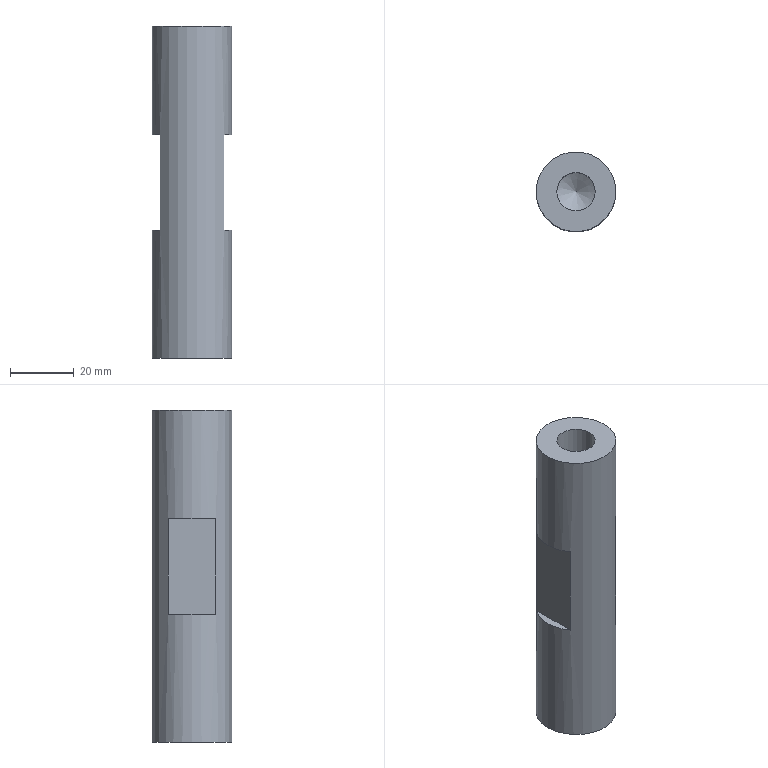Part | NX | features solid 2 | 1 solid | 13 faces | box 25 x 25 x 104 mm | volume 43591 mm3 | plane 8 | cylinder 3 | cone 2 | commonest cylinder face diameters 12 x2 25 x1
STEP:
#1=CARTESIAN_POINT('',(-537.5,-40.,-65.));
#2=VERTEX_POINT('',#1);
#3=CARTESIAN_POINT('',(-525.,-40.,-65.));
#4=DIRECTION('',(0.,0.,-1.));
#5=DIRECTION('',(-1.,0.,0.));
#6=AXIS2_PLACEMENT_3D('',#3,#4,#5);
#7=CIRCLE('',#6,12.5);
#8=EDGE_CURVE('',#2,#2,#7,.F.);
#9=ORIENTED_EDGE('',*,*,#8,.F.);
#10=EDGE_LOOP('',(#9));
#11=FACE_BOUND('',#10,.T.);
#12=CARTESIAN_POINT('',(-512.5,-40.,-169.));
#13=VERTEX_POINT('',#12);
#14=CARTESIAN_POINT('',(-525.,-40.,-169.));
#15=DIRECTION('',(0.,0.,1.));
#16=DIRECTION('',(1.,0.,0.));
#17=AXIS2_PLACEMENT_3D('',#14,#15,#16);
#18=CIRCLE('',#17,12.5);
#19=EDGE_CURVE('',#13,#13,#18,.T.);
#20=ORIENTED_EDGE('',*,*,#19,.T.);
#21=EDGE_LOOP('',(#20));
#22=FACE_BOUND('',#21,.T.);
#23=CARTESIAN_POINT('',(-515.,-47.5,-99.));
#24=VERTEX_POINT('',#23);
#25=CARTESIAN_POINT('',(-515.,-47.5,-129.));
#26=VERTEX_POINT('',#25);
#27=CARTESIAN_POINT('',(-515.,-47.5,-169.));
#28=DIRECTION('',(0.,0.,1.));
#29=VECTOR('',#28,1000.);
#30=LINE('',#27,#29);
#31=EDGE_CURVE('',#24,#26,#30,.F.);
#32=ORIENTED_EDGE('',*,*,#31,.F.);
#33=CARTESIAN_POINT('',(-515.,-32.5,-99.));
#34=VERTEX_POINT('',#33);
#35=CARTESIAN_POINT('',(-525.,-40.,-99.));
#36=DIRECTION('',(0.,0.,-1.));
#37=DIRECTION('',(-1.,0.,0.));
#38=AXIS2_PLACEMENT_3D('',#35,#36,#37);
#39=CIRCLE('',#38,12.5);
#40=EDGE_CURVE('',#34,#24,#39,.T.);
#41=ORIENTED_EDGE('',*,*,#40,.F.);
#42=CARTESIAN_POINT('',(-515.,-32.5,-129.));
#43=VERTEX_POINT('',#42);
#44=CARTESIAN_POINT('',(-515.,-32.5,-169.));
#45=DIRECTION('',(0.,0.,1.));
#46=VECTOR('',#45,1000.);
#47=LINE('',#44,#46);
#48=EDGE_CURVE('',#43,#34,#47,.T.);
#49=ORIENTED_EDGE('',*,*,#48,.F.);
#50=CARTESIAN_POINT('',(-525.,-40.,-129.));
#51=DIRECTION('',(0.,0.,-1.));
#52=DIRECTION('',(-1.,0.,0.));
#53=AXIS2_PLACEMENT_3D('',#50,#51,#52);
#54=CIRCLE('',#53,12.5);
#55=EDGE_CURVE('',#26,#43,#54,.F.);
#56=ORIENTED_EDGE('',*,*,#55,.F.);
#57=EDGE_LOOP('',(#32,#41,#49,#56));
#58=FACE_BOUND('',#57,.T.);
#59=CARTESIAN_POINT('',(-535.,-32.5,-99.));
#60=VERTEX_POINT('',#59);
#61=CARTESIAN_POINT('',(-535.,-47.5,-99.));
#62=VERTEX_POINT('',#61);
#63=CARTESIAN_POINT('',(-525.,-40.,-99.));
#64=DIRECTION('',(0.,0.,-1.));
#65=DIRECTION('',(-1.,0.,0.));
#66=AXIS2_PLACEMENT_3D('',#63,#64,#65);
#67=CIRCLE('',#66,12.5);
#68=EDGE_CURVE('',#60,#62,#67,.F.);
#69=ORIENTED_EDGE('',*,*,#68,.T.);
#70=CARTESIAN_POINT('',(-535.,-47.5,-129.));
#71=VERTEX_POINT('',#70);
#72=CARTESIAN_POINT('',(-535.,-47.5,-99.));
#73=DIRECTION('',(0.,0.,1.));
#74=VECTOR('',#73,1000.);
#75=LINE('',#72,#74);
#76=EDGE_CURVE('',#62,#71,#75,.F.);
#77=ORIENTED_EDGE('',*,*,#76,.T.);
#78=CARTESIAN_POINT('',(-535.,-32.5,-129.));
#79=VERTEX_POINT('',#78);
#80=CARTESIAN_POINT('',(-525.,-40.,-129.));
#81=DIRECTION('',(0.,0.,-1.));
#82=DIRECTION('',(-1.,0.,0.));
#83=AXIS2_PLACEMENT_3D('',#80,#81,#82);
#84=CIRCLE('',#83,12.5);
#85=EDGE_CURVE('',#71,#79,#84,.T.);
#86=ORIENTED_EDGE('',*,*,#85,.T.);
#87=CARTESIAN_POINT('',(-535.,-32.5,-169.));
#88=DIRECTION('',(0.,0.,1.));
#89=VECTOR('',#88,1000.);
#90=LINE('',#87,#89);
#91=EDGE_CURVE('',#79,#60,#90,.T.);
#92=ORIENTED_EDGE('',*,*,#91,.T.);
#93=EDGE_LOOP('',(#69,#77,#86,#92));
#94=FACE_BOUND('',#93,.T.);
#95=CARTESIAN_POINT('',(-525.,-40.,-169.));
#96=DIRECTION('',(0.,0.,1.));
#97=DIRECTION('',(1.,0.,0.));
#98=AXIS2_PLACEMENT_3D('',#95,#96,#97);
#99=CYLINDRICAL_SURFACE('',#98,12.5);
#100=ADVANCED_FACE('',(#11,#22,#58,#94),#99,.T.);
#101=CARTESIAN_POINT('',(-519.,-40.,-169.));
#102=VERTEX_POINT('',#101);
#103=CARTESIAN_POINT('',(-525.,-40.,-169.));
#104=DIRECTION('',(0.,0.,1.));
#105=DIRECTION('',(1.,0.,0.));
#106=AXIS2_PLACEMENT_3D('',#103,#104,#105);
#107=CIRCLE('',#106,6.);
#108=EDGE_CURVE('',#102,#102,#107,.T.);
#109=ORIENTED_EDGE('',*,*,#108,.T.);
#110=EDGE_LOOP('',(#109));
#111=FACE_BOUND('',#110,.T.);
#112=ORIENTED_EDGE('',*,*,#19,.F.);
#113=EDGE_LOOP('',(#112));
#114=FACE_BOUND('',#113,.T.);
#115=CARTESIAN_POINT('',(-525.,-40.,-169.));
#116=DIRECTION('',(0.,0.,1.));
#117=DIRECTION('',(1.,0.,0.));
#118=AXIS2_PLACEMENT_3D('',#115,#116,#117);
#119=PLANE('',#118);
#120=ADVANCED_FACE('',(#111,#114),#119,.F.);
#121=CARTESIAN_POINT('',(-531.,-40.,-65.));
#122=VERTEX_POINT('',#121);
#123=CARTESIAN_POINT('',(-525.,-40.,-65.));
#124=DIRECTION('',(0.,0.,-1.));
#125=DIRECTION('',(-1.,0.,0.));
#126=AXIS2_PLACEMENT_3D('',#123,#124,#125);
#127=CIRCLE('',#126,6.);
#128=EDGE_CURVE('',#122,#122,#127,.T.);
#129=ORIENTED_EDGE('',*,*,#128,.T.);
#130=EDGE_LOOP('',(#129));
#131=FACE_BOUND('',#130,.T.);
#132=ORIENTED_EDGE('',*,*,#8,.T.);
#133=EDGE_LOOP('',(#132));
#134=FACE_BOUND('',#133,.T.);
#135=CARTESIAN_POINT('',(-610.,110.,-65.));
#136=DIRECTION('',(0.,0.,-1.));
#137=DIRECTION('',(0.,1.,0.));
#138=AXIS2_PLACEMENT_3D('',#135,#136,#137);
#139=PLANE('',#138);
#140=ADVANCED_FACE('',(#131,#134),#139,.F.);
#141=CARTESIAN_POINT('',(-531.,-40.,-85.));
#142=VERTEX_POINT('',#141);
#143=CARTESIAN_POINT('',(-525.,-40.,-85.));
#144=DIRECTION('',(0.,0.,-1.));
#145=DIRECTION('',(-1.,0.,0.));
#146=AXIS2_PLACEMENT_3D('',#143,#144,#145);
#147=CIRCLE('',#146,6.);
#148=EDGE_CURVE('',#142,#142,#147,.T.);
#149=ORIENTED_EDGE('',*,*,#148,.F.);
#150=EDGE_LOOP('',(#149));
#151=FACE_BOUND('',#150,.T.);
#152=CARTESIAN_POINT('',(-525.,-40.,-88.605));
#153=VERTEX_POINT('',#152);
#154=VERTEX_LOOP('',#153);
#155=FACE_BOUND('',#154,.T.);
#156=CARTESIAN_POINT('',(-525.,-40.,-85.));
#157=DIRECTION('',(0.,0.,1.));
#158=DIRECTION('',(1.,0.,0.));
#159=AXIS2_PLACEMENT_3D('',#156,#157,#158);
#160=CONICAL_SURFACE('',#159,6.,1.03);
#161=ADVANCED_FACE('',(#151,#155),#160,.F.);
#162=ORIENTED_EDGE('',*,*,#148,.T.);
#163=EDGE_LOOP('',(#162));
#164=FACE_BOUND('',#163,.T.);
#165=ORIENTED_EDGE('',*,*,#128,.F.);
#166=EDGE_LOOP('',(#165));
#167=FACE_BOUND('',#166,.T.);
#168=CARTESIAN_POINT('',(-525.,-40.,-65.));
#169=DIRECTION('',(0.,0.,-1.));
#170=DIRECTION('',(-1.,0.,0.));
#171=AXIS2_PLACEMENT_3D('',#168,#169,#170);
#172=CYLINDRICAL_SURFACE('',#171,6.);
#173=ADVANCED_FACE('',(#164,#167),#172,.F.);
#174=CARTESIAN_POINT('',(-519.,-40.,-139.));
#175=VERTEX_POINT('',#174);
#176=CARTESIAN_POINT('',(-525.,-40.,-139.));
#177=DIRECTION('',(0.,0.,1.));
#178=DIRECTION('',(1.,0.,0.));
#179=AXIS2_PLACEMENT_3D('',#176,#177,#178);
#180=CIRCLE('',#179,6.);
#181=EDGE_CURVE('',#175,#175,#180,.T.);
#182=ORIENTED_EDGE('',*,*,#181,.F.);
#183=EDGE_LOOP('',(#182));
#184=FACE_BOUND('',#183,.T.);
#185=CARTESIAN_POINT('',(-525.,-40.,-135.395));
#186=VERTEX_POINT('',#185);
#187=VERTEX_LOOP('',#186);
#188=FACE_BOUND('',#187,.T.);
#189=CARTESIAN_POINT('',(-525.,-40.,-139.));
#190=DIRECTION('',(0.,0.,-1.));
#191=DIRECTION('',(-1.,0.,0.));
#192=AXIS2_PLACEMENT_3D('',#189,#190,#191);
#193=CONICAL_SURFACE('',#192,6.,1.03);
#194=ADVANCED_FACE('',(#184,#188),#193,.F.);
#195=ORIENTED_EDGE('',*,*,#181,.T.);
#196=EDGE_LOOP('',(#195));
#197=FACE_BOUND('',#196,.T.);
#198=ORIENTED_EDGE('',*,*,#108,.F.);
#199=EDGE_LOOP('',(#198));
#200=FACE_BOUND('',#199,.T.);
#201=CARTESIAN_POINT('',(-525.,-40.,-169.));
#202=DIRECTION('',(0.,0.,1.));
#203=DIRECTION('',(1.,0.,0.));
#204=AXIS2_PLACEMENT_3D('',#201,#202,#203);
#205=CYLINDRICAL_SURFACE('',#204,6.);
#206=ADVANCED_FACE('',(#197,#200),#205,.F.);
#207=ORIENTED_EDGE('',*,*,#55,.T.);
#208=CARTESIAN_POINT('',(-515.,-25.,-129.));
#209=DIRECTION('',(0.,-1.,0.));
#210=VECTOR('',#209,1000.);
#211=LINE('',#208,#210);
#212=EDGE_CURVE('',#43,#26,#211,.T.);
#213=ORIENTED_EDGE('',*,*,#212,.T.);
#214=EDGE_LOOP('',(#207,#213));
#215=FACE_BOUND('',#214,.T.);
#216=CARTESIAN_POINT('',(-525.,-25.,-129.));
#217=DIRECTION('',(0.,0.,-1.));
#218=DIRECTION('',(0.,-1.,0.));
#219=AXIS2_PLACEMENT_3D('',#216,#217,#218);
#220=PLANE('',#219);
#221=ADVANCED_FACE('',(#215),#220,.F.);
#222=ORIENTED_EDGE('',*,*,#40,.T.);
#223=CARTESIAN_POINT('',(-515.,-25.,-99.));
#224=DIRECTION('',(0.,1.,0.));
#225=VECTOR('',#224,1000.);
#226=LINE('',#223,#225);
#227=EDGE_CURVE('',#34,#24,#226,.F.);
#228=ORIENTED_EDGE('',*,*,#227,.F.);
#229=EDGE_LOOP('',(#222,#228));
#230=FACE_BOUND('',#229,.T.);
#231=CARTESIAN_POINT('',(-525.,-25.,-99.));
#232=DIRECTION('',(0.,0.,-1.));
#233=DIRECTION('',(0.,-1.,0.));
#234=AXIS2_PLACEMENT_3D('',#231,#232,#233);
#235=PLANE('',#234);
#236=ADVANCED_FACE('',(#230),#235,.T.);
#237=ORIENTED_EDGE('',*,*,#31,.T.);
#238=ORIENTED_EDGE('',*,*,#212,.F.);
#239=ORIENTED_EDGE('',*,*,#48,.T.);
#240=ORIENTED_EDGE('',*,*,#227,.T.);
#241=EDGE_LOOP('',(#237,#238,#239,#240));
#242=FACE_BOUND('',#241,.T.);
#243=CARTESIAN_POINT('',(-515.,-25.,-129.));
#244=DIRECTION('',(-1.,0.,0.));
#245=DIRECTION('',(0.,0.,1.));
#246=AXIS2_PLACEMENT_3D('',#243,#244,#245);
#247=PLANE('',#246);
#248=ADVANCED_FACE('',(#242),#247,.F.);
#249=CARTESIAN_POINT('',(-535.,-25.,-129.));
#250=DIRECTION('',(0.,1.,0.));
#251=VECTOR('',#250,1000.);
#252=LINE('',#249,#251);
#253=EDGE_CURVE('',#79,#71,#252,.F.);
#254=ORIENTED_EDGE('',*,*,#253,.F.);
#255=ORIENTED_EDGE('',*,*,#85,.F.);
#256=EDGE_LOOP('',(#254,#255));
#257=FACE_BOUND('',#256,.T.);
#258=CARTESIAN_POINT('',(-525.,-25.,-129.));
#259=DIRECTION('',(0.,0.,-1.));
#260=DIRECTION('',(0.,-1.,0.));
#261=AXIS2_PLACEMENT_3D('',#258,#259,#260);
#262=PLANE('',#261);
#263=ADVANCED_FACE('',(#257),#262,.F.);
#264=CARTESIAN_POINT('',(-535.,-25.,-99.));
#265=DIRECTION('',(0.,-1.,0.));
#266=VECTOR('',#265,1000.);
#267=LINE('',#264,#266);
#268=EDGE_CURVE('',#60,#62,#267,.T.);
#269=ORIENTED_EDGE('',*,*,#268,.T.);
#270=ORIENTED_EDGE('',*,*,#68,.F.);
#271=EDGE_LOOP('',(#269,#270));
#272=FACE_BOUND('',#271,.T.);
#273=CARTESIAN_POINT('',(-525.,-25.,-99.));
#274=DIRECTION('',(0.,0.,-1.));
#275=DIRECTION('',(0.,-1.,0.));
#276=AXIS2_PLACEMENT_3D('',#273,#274,#275);
#277=PLANE('',#276);
#278=ADVANCED_FACE('',(#272),#277,.T.);
#279=ORIENTED_EDGE('',*,*,#268,.F.);
#280=ORIENTED_EDGE('',*,*,#91,.F.);
#281=ORIENTED_EDGE('',*,*,#253,.T.);
#282=ORIENTED_EDGE('',*,*,#76,.F.);
#283=EDGE_LOOP('',(#279,#280,#281,#282));
#284=FACE_BOUND('',#283,.T.);
#285=CARTESIAN_POINT('',(-535.,-25.,-129.));
#286=DIRECTION('',(-1.,0.,0.));
#287=DIRECTION('',(0.,0.,1.));
#288=AXIS2_PLACEMENT_3D('',#285,#286,#287);
#289=PLANE('',#288);
#290=ADVANCED_FACE('',(#284),#289,.T.);
#291=CLOSED_SHELL('',(#100,#120,#140,#161,#173,#194,#206,#221,#236,#248,#263,#278,#290));
#292=MANIFOLD_SOLID_BREP('',#291);
#293=(LENGTH_UNIT()NAMED_UNIT(*)SI_UNIT(.MILLI.,.METRE.));
#294=UNCERTAINTY_MEASURE_WITH_UNIT(LENGTH_MEASURE(0.00001),#293,'','');
#295=(NAMED_UNIT(*)PLANE_ANGLE_UNIT()SI_UNIT($,.RADIAN.));
#296=(NAMED_UNIT(*)SI_UNIT($,.STERADIAN.)SOLID_ANGLE_UNIT());
#297=(GEOMETRIC_REPRESENTATION_CONTEXT(3)GLOBAL_UNCERTAINTY_ASSIGNED_CONTEXT((#294))GLOBAL_UNIT_ASSIGNED_CONTEXT((#293,#295,#296))REPRESENTATION_CONTEXT('',''));
#298=ADVANCED_BREP_SHAPE_REPRESENTATION('',(#292),#297);